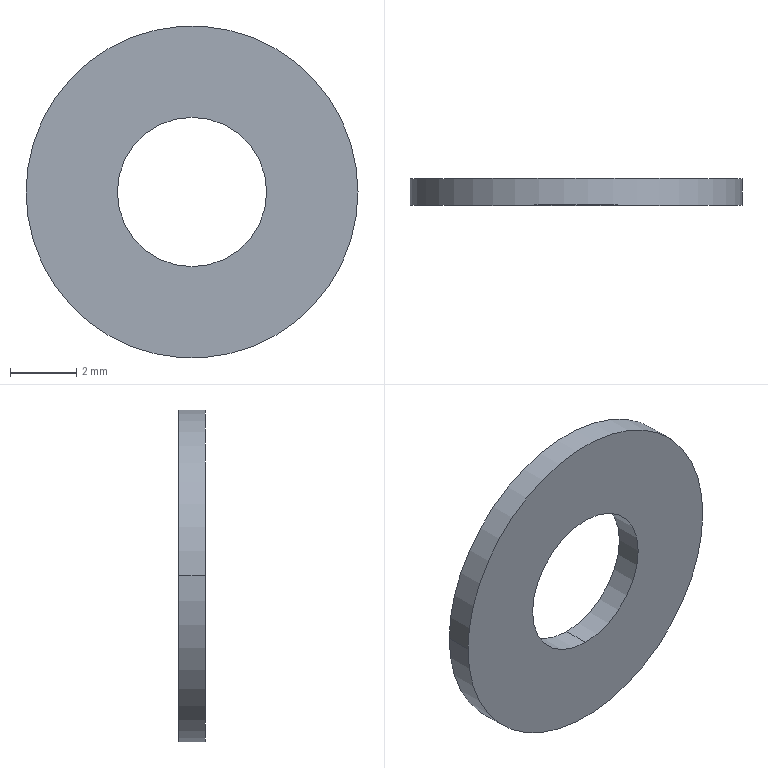Part | STEP file | ZZ21-M4-8 | 1 solid | 6 faces | box 10 x 0.8 x 10 mm | volume 50.108 mm3 | cylinder 4 | plane 2 | commonest cylinder face diameters 4.5 x2 10 x2
STEP:
#1=CARTESIAN_POINT('',(0.,0.,0.));
#2=DIRECTION('',(0.,0.,1.));
#3=DIRECTION('',(1.,0.,0.));
#4=AXIS2_PLACEMENT_3D('',#1,#2,#3);
#5=CARTESIAN_POINT('',(0.,0.,-2.25));
#6=VERTEX_POINT('',#5);
#7=CARTESIAN_POINT('',(0.,0.8,-2.25));
#8=VERTEX_POINT('',#7);
#9=CARTESIAN_POINT('',(0.,0.,-2.25));
#10=DIRECTION('',(0.,1.,0.));
#11=VECTOR('',#10,1.);
#12=LINE('',#9,#11);
#13=CARTESIAN_POINT('',(0.,0.,0.));
#14=DIRECTION('',(0.,1.,0.));
#15=DIRECTION('',(0.,0.,-1.));
#16=AXIS2_PLACEMENT_3D('',#13,#14,#15);
#17=CYLINDRICAL_SURFACE('',#16,2.25);
#18=CARTESIAN_POINT('',(6.283,0.));
#19=DIRECTION('',(0.,1.));
#20=VECTOR('',#19,1.);
#21=LINE('',#18,#20);
#22=(GEOMETRIC_REPRESENTATION_CONTEXT(2)PARAMETRIC_REPRESENTATION_CONTEXT()REPRESENTATION_CONTEXT('',''));
#23=DEFINITIONAL_REPRESENTATION('',(#21),#22);
#24=PCURVE('',#17,#23);
#25=CARTESIAN_POINT('',(0.,0.,0.));
#26=DIRECTION('',(0.,1.,0.));
#27=DIRECTION('',(0.,0.,-1.));
#28=AXIS2_PLACEMENT_3D('',#25,#26,#27);
#29=CYLINDRICAL_SURFACE('',#28,2.25);
#30=CARTESIAN_POINT('',(0.,0.));
#31=DIRECTION('',(0.,1.));
#32=VECTOR('',#31,1.);
#33=LINE('',#30,#32);
#34=(GEOMETRIC_REPRESENTATION_CONTEXT(2)PARAMETRIC_REPRESENTATION_CONTEXT()REPRESENTATION_CONTEXT('',''));
#35=DEFINITIONAL_REPRESENTATION('',(#33),#34);
#36=PCURVE('',#29,#35);
#37=SURFACE_CURVE('',#12,(#24,#36),.PCURVE_S1.);
#38=EDGE_CURVE('',#6,#8,#37,.T.);
#39=ORIENTED_EDGE('',*,*,#38,.T.);
#40=CARTESIAN_POINT('',(0.,0.8,2.25));
#41=VERTEX_POINT('',#40);
#42=CARTESIAN_POINT('',(0.,0.8,0.));
#43=DIRECTION('',(0.,-1.,0.));
#44=DIRECTION('',(0.,0.,1.));
#45=AXIS2_PLACEMENT_3D('',#42,#43,#44);
#46=CIRCLE('',#45,2.25);
#47=CARTESIAN_POINT('',(9.425,0.8));
#48=DIRECTION('',(-1.,0.));
#49=VECTOR('',#48,1.);
#50=LINE('',#47,#49);
#51=(GEOMETRIC_REPRESENTATION_CONTEXT(2)PARAMETRIC_REPRESENTATION_CONTEXT()REPRESENTATION_CONTEXT('',''));
#52=DEFINITIONAL_REPRESENTATION('',(#50),#51);
#53=PCURVE('',#17,#52);
#54=CARTESIAN_POINT('',(0.,0.8,0.));
#55=DIRECTION('',(0.,1.,0.));
#56=DIRECTION('',(-1.,0.,0.));
#57=AXIS2_PLACEMENT_3D('',#54,#55,#56);
#58=PLANE('',#57);
#59=CARTESIAN_POINT('',(0.,2.25));
#60=CARTESIAN_POINT('',(3.897,2.25));
#61=CARTESIAN_POINT('',(1.949,-1.125));
#62=CARTESIAN_POINT('',(0.,-4.5));
#63=CARTESIAN_POINT('',(-1.949,-1.125));
#64=CARTESIAN_POINT('',(-3.897,2.25));
#65=CARTESIAN_POINT('',(0.,2.25));
#66=(BOUNDED_CURVE()B_SPLINE_CURVE(2,(#59,#60,#61,#62,#63,#64,#65),.UNSPECIFIED.,.T.,.F.)B_SPLINE_CURVE_WITH_KNOTS((1,2,2,2,2,1),(-2.094,0.,2.094,4.189,6.283,8.378),.UNSPECIFIED.)CURVE()GEOMETRIC_REPRESENTATION_ITEM()RATIONAL_B_SPLINE_CURVE((1.,0.5,1.,0.5,1.,0.5,1.))REPRESENTATION_ITEM(''));
#67=(GEOMETRIC_REPRESENTATION_CONTEXT(2)PARAMETRIC_REPRESENTATION_CONTEXT()REPRESENTATION_CONTEXT('',''));
#68=DEFINITIONAL_REPRESENTATION('',(#66),#67);
#69=PCURVE('',#58,#68);
#70=SURFACE_CURVE('',#46,(#53,#69),.PCURVE_S1.);
#71=EDGE_CURVE('',#8,#41,#70,.T.);
#72=ORIENTED_EDGE('',*,*,#71,.T.);
#73=CARTESIAN_POINT('',(0.,0.,2.25));
#74=VERTEX_POINT('',#73);
#75=CARTESIAN_POINT('',(0.,0.,2.25));
#76=DIRECTION('',(0.,1.,0.));
#77=VECTOR('',#76,1.);
#78=LINE('',#75,#77);
#79=CARTESIAN_POINT('',(3.142,0.));
#80=DIRECTION('',(0.,1.));
#81=VECTOR('',#80,1.);
#82=LINE('',#79,#81);
#83=(GEOMETRIC_REPRESENTATION_CONTEXT(2)PARAMETRIC_REPRESENTATION_CONTEXT()REPRESENTATION_CONTEXT('',''));
#84=DEFINITIONAL_REPRESENTATION('',(#82),#83);
#85=PCURVE('',#17,#84);
#86=CARTESIAN_POINT('',(3.142,0.));
#87=DIRECTION('',(0.,1.));
#88=VECTOR('',#87,1.);
#89=LINE('',#86,#88);
#90=(GEOMETRIC_REPRESENTATION_CONTEXT(2)PARAMETRIC_REPRESENTATION_CONTEXT()REPRESENTATION_CONTEXT('',''));
#91=DEFINITIONAL_REPRESENTATION('',(#89),#90);
#92=PCURVE('',#29,#91);
#93=SURFACE_CURVE('',#78,(#85,#92),.PCURVE_S1.);
#94=EDGE_CURVE('',#74,#41,#93,.T.);
#95=ORIENTED_EDGE('',*,*,#94,.F.);
#96=CARTESIAN_POINT('',(0.,0.,0.));
#97=DIRECTION('',(0.,1.,0.));
#98=DIRECTION('',(0.,0.,-1.));
#99=AXIS2_PLACEMENT_3D('',#96,#97,#98);
#100=CIRCLE('',#99,2.25);
#101=CARTESIAN_POINT('',(0.,0.));
#102=DIRECTION('',(1.,0.));
#103=VECTOR('',#102,1.);
#104=LINE('',#101,#103);
#105=(GEOMETRIC_REPRESENTATION_CONTEXT(2)PARAMETRIC_REPRESENTATION_CONTEXT()REPRESENTATION_CONTEXT('',''));
#106=DEFINITIONAL_REPRESENTATION('',(#104),#105);
#107=PCURVE('',#17,#106);
#108=CARTESIAN_POINT('',(0.,0.,0.));
#109=DIRECTION('',(0.,-1.,0.));
#110=DIRECTION('',(1.,0.,0.));
#111=AXIS2_PLACEMENT_3D('',#108,#109,#110);
#112=PLANE('',#111);
#113=CARTESIAN_POINT('',(0.,-2.25));
#114=CARTESIAN_POINT('',(-3.897,-2.25));
#115=CARTESIAN_POINT('',(-1.949,1.125));
#116=CARTESIAN_POINT('',(0.,4.5));
#117=CARTESIAN_POINT('',(1.949,1.125));
#118=CARTESIAN_POINT('',(3.897,-2.25));
#119=CARTESIAN_POINT('',(0.,-2.25));
#120=(BOUNDED_CURVE()B_SPLINE_CURVE(2,(#113,#114,#115,#116,#117,#118,#119),.UNSPECIFIED.,.T.,.F.)B_SPLINE_CURVE_WITH_KNOTS((1,2,2,2,2,1),(-2.094,0.,2.094,4.189,6.283,8.378),.UNSPECIFIED.)CURVE()GEOMETRIC_REPRESENTATION_ITEM()RATIONAL_B_SPLINE_CURVE((1.,0.5,1.,0.5,1.,0.5,1.))REPRESENTATION_ITEM(''));
#121=(GEOMETRIC_REPRESENTATION_CONTEXT(2)PARAMETRIC_REPRESENTATION_CONTEXT()REPRESENTATION_CONTEXT('',''));
#122=DEFINITIONAL_REPRESENTATION('',(#120),#121);
#123=PCURVE('',#112,#122);
#124=SURFACE_CURVE('',#100,(#107,#123),.PCURVE_S1.);
#125=EDGE_CURVE('',#74,#6,#124,.T.);
#126=ORIENTED_EDGE('',*,*,#125,.T.);
#127=EDGE_LOOP('',(#39,#72,#95,#126));
#128=FACE_BOUND('',#127,.F.);
#129=ADVANCED_FACE('',(#128),#17,.F.);
#130=CARTESIAN_POINT('',(-5.,0.,0.));
#131=VERTEX_POINT('',#130);
#132=CARTESIAN_POINT('',(5.,0.,0.));
#133=VERTEX_POINT('',#132);
#134=CARTESIAN_POINT('',(0.,0.,0.));
#135=DIRECTION('',(0.,1.,0.));
#136=DIRECTION('',(-1.,0.,0.));
#137=AXIS2_PLACEMENT_3D('',#134,#135,#136);
#138=CIRCLE('',#137,5.);
#139=CARTESIAN_POINT('',(0.,0.,0.));
#140=DIRECTION('',(0.,1.,0.));
#141=DIRECTION('',(-1.,0.,0.));
#142=AXIS2_PLACEMENT_3D('',#139,#140,#141);
#143=CYLINDRICAL_SURFACE('',#142,5.);
#144=CARTESIAN_POINT('',(0.,0.));
#145=DIRECTION('',(1.,0.));
#146=VECTOR('',#145,1.);
#147=LINE('',#144,#146);
#148=(GEOMETRIC_REPRESENTATION_CONTEXT(2)PARAMETRIC_REPRESENTATION_CONTEXT()REPRESENTATION_CONTEXT('',''));
#149=DEFINITIONAL_REPRESENTATION('',(#147),#148);
#150=PCURVE('',#143,#149);
#151=CARTESIAN_POINT('',(-5.,0.));
#152=CARTESIAN_POINT('',(-5.,8.66));
#153=CARTESIAN_POINT('',(2.5,4.33));
#154=CARTESIAN_POINT('',(10.,0.));
#155=CARTESIAN_POINT('',(2.5,-4.33));
#156=CARTESIAN_POINT('',(-5.,-8.66));
#157=CARTESIAN_POINT('',(-5.,0.));
#158=(BOUNDED_CURVE()B_SPLINE_CURVE(2,(#151,#152,#153,#154,#155,#156,#157),.UNSPECIFIED.,.T.,.F.)B_SPLINE_CURVE_WITH_KNOTS((1,2,2,2,2,1),(-2.094,0.,2.094,4.189,6.283,8.378),.UNSPECIFIED.)CURVE()GEOMETRIC_REPRESENTATION_ITEM()RATIONAL_B_SPLINE_CURVE((1.,0.5,1.,0.5,1.,0.5,1.))REPRESENTATION_ITEM(''));
#159=(GEOMETRIC_REPRESENTATION_CONTEXT(2)PARAMETRIC_REPRESENTATION_CONTEXT()REPRESENTATION_CONTEXT('',''));
#160=DEFINITIONAL_REPRESENTATION('',(#158),#159);
#161=PCURVE('',#112,#160);
#162=SURFACE_CURVE('',#138,(#150,#161),.PCURVE_S1.);
#163=EDGE_CURVE('',#131,#133,#162,.T.);
#164=ORIENTED_EDGE('',*,*,#163,.T.);
#165=CARTESIAN_POINT('',(5.,0.8,0.));
#166=VERTEX_POINT('',#165);
#167=CARTESIAN_POINT('',(5.,0.,0.));
#168=DIRECTION('',(0.,1.,0.));
#169=VECTOR('',#168,1.);
#170=LINE('',#167,#169);
#171=CARTESIAN_POINT('',(3.142,0.));
#172=DIRECTION('',(0.,1.));
#173=VECTOR('',#172,1.);
#174=LINE('',#171,#173);
#175=(GEOMETRIC_REPRESENTATION_CONTEXT(2)PARAMETRIC_REPRESENTATION_CONTEXT()REPRESENTATION_CONTEXT('',''));
#176=DEFINITIONAL_REPRESENTATION('',(#174),#175);
#177=PCURVE('',#143,#176);
#178=CARTESIAN_POINT('',(0.,0.,0.));
#179=DIRECTION('',(0.,1.,0.));
#180=DIRECTION('',(-1.,0.,0.));
#181=AXIS2_PLACEMENT_3D('',#178,#179,#180);
#182=CYLINDRICAL_SURFACE('',#181,5.);
#183=CARTESIAN_POINT('',(3.142,0.));
#184=DIRECTION('',(0.,1.));
#185=VECTOR('',#184,1.);
#186=LINE('',#183,#185);
#187=(GEOMETRIC_REPRESENTATION_CONTEXT(2)PARAMETRIC_REPRESENTATION_CONTEXT()REPRESENTATION_CONTEXT('',''));
#188=DEFINITIONAL_REPRESENTATION('',(#186),#187);
#189=PCURVE('',#182,#188);
#190=SURFACE_CURVE('',#170,(#177,#189),.PCURVE_S1.);
#191=EDGE_CURVE('',#133,#166,#190,.T.);
#192=ORIENTED_EDGE('',*,*,#191,.T.);
#193=CARTESIAN_POINT('',(-5.,0.8,0.));
#194=VERTEX_POINT('',#193);
#195=CARTESIAN_POINT('',(0.,0.8,0.));
#196=DIRECTION('',(0.,-1.,0.));
#197=DIRECTION('',(1.,0.,0.));
#198=AXIS2_PLACEMENT_3D('',#195,#196,#197);
#199=CIRCLE('',#198,5.);
#200=CARTESIAN_POINT('',(3.142,0.8));
#201=DIRECTION('',(-1.,0.));
#202=VECTOR('',#201,1.);
#203=LINE('',#200,#202);
#204=(GEOMETRIC_REPRESENTATION_CONTEXT(2)PARAMETRIC_REPRESENTATION_CONTEXT()REPRESENTATION_CONTEXT('',''));
#205=DEFINITIONAL_REPRESENTATION('',(#203),#204);
#206=PCURVE('',#143,#205);
#207=CARTESIAN_POINT('',(-5.,0.));
#208=CARTESIAN_POINT('',(-5.,8.66));
#209=CARTESIAN_POINT('',(2.5,4.33));
#210=CARTESIAN_POINT('',(10.,0.));
#211=CARTESIAN_POINT('',(2.5,-4.33));
#212=CARTESIAN_POINT('',(-5.,-8.66));
#213=CARTESIAN_POINT('',(-5.,0.));
#214=(BOUNDED_CURVE()B_SPLINE_CURVE(2,(#207,#208,#209,#210,#211,#212,#213),.UNSPECIFIED.,.T.,.F.)B_SPLINE_CURVE_WITH_KNOTS((1,2,2,2,2,1),(-2.094,0.,2.094,4.189,6.283,8.378),.UNSPECIFIED.)CURVE()GEOMETRIC_REPRESENTATION_ITEM()RATIONAL_B_SPLINE_CURVE((1.,0.5,1.,0.5,1.,0.5,1.))REPRESENTATION_ITEM(''));
#215=(GEOMETRIC_REPRESENTATION_CONTEXT(2)PARAMETRIC_REPRESENTATION_CONTEXT()REPRESENTATION_CONTEXT('',''));
#216=DEFINITIONAL_REPRESENTATION('',(#214),#215);
#217=PCURVE('',#58,#216);
#218=SURFACE_CURVE('',#199,(#206,#217),.PCURVE_S1.);
#219=EDGE_CURVE('',#166,#194,#218,.T.);
#220=ORIENTED_EDGE('',*,*,#219,.T.);
#221=CARTESIAN_POINT('',(-5.,0.,0.));
#222=DIRECTION('',(0.,1.,0.));
#223=VECTOR('',#222,1.);
#224=LINE('',#221,#223);
#225=CARTESIAN_POINT('',(0.,0.));
#226=DIRECTION('',(0.,1.));
#227=VECTOR('',#226,1.);
#228=LINE('',#225,#227);
#229=(GEOMETRIC_REPRESENTATION_CONTEXT(2)PARAMETRIC_REPRESENTATION_CONTEXT()REPRESENTATION_CONTEXT('',''));
#230=DEFINITIONAL_REPRESENTATION('',(#228),#229);
#231=PCURVE('',#143,#230);
#232=CARTESIAN_POINT('',(6.283,0.));
#233=DIRECTION('',(0.,1.));
#234=VECTOR('',#233,1.);
#235=LINE('',#232,#234);
#236=(GEOMETRIC_REPRESENTATION_CONTEXT(2)PARAMETRIC_REPRESENTATION_CONTEXT()REPRESENTATION_CONTEXT('',''));
#237=DEFINITIONAL_REPRESENTATION('',(#235),#236);
#238=PCURVE('',#182,#237);
#239=SURFACE_CURVE('',#224,(#231,#238),.PCURVE_S1.);
#240=EDGE_CURVE('',#131,#194,#239,.T.);
#241=ORIENTED_EDGE('',*,*,#240,.F.);
#242=EDGE_LOOP('',(#164,#192,#220,#241));
#243=FACE_BOUND('',#242,.T.);
#244=ADVANCED_FACE('',(#243),#143,.T.);
#245=ORIENTED_EDGE('',*,*,#71,.T.);
#246=CARTESIAN_POINT('',(0.,0.8,0.));
#247=DIRECTION('',(0.,-1.,0.));
#248=DIRECTION('',(0.,0.,1.));
#249=AXIS2_PLACEMENT_3D('',#246,#247,#248);
#250=CIRCLE('',#249,2.25);
#251=CARTESIAN_POINT('',(0.,2.25));
#252=CARTESIAN_POINT('',(3.897,2.25));
#253=CARTESIAN_POINT('',(1.949,-1.125));
#254=CARTESIAN_POINT('',(0.,-4.5));
#255=CARTESIAN_POINT('',(-1.949,-1.125));
#256=CARTESIAN_POINT('',(-3.897,2.25));
#257=CARTESIAN_POINT('',(0.,2.25));
#258=(BOUNDED_CURVE()B_SPLINE_CURVE(2,(#251,#252,#253,#254,#255,#256,#257),.UNSPECIFIED.,.T.,.F.)B_SPLINE_CURVE_WITH_KNOTS((1,2,2,2,2,1),(-2.094,0.,2.094,4.189,6.283,8.378),.UNSPECIFIED.)CURVE()GEOMETRIC_REPRESENTATION_ITEM()RATIONAL_B_SPLINE_CURVE((1.,0.5,1.,0.5,1.,0.5,1.))REPRESENTATION_ITEM(''));
#259=(GEOMETRIC_REPRESENTATION_CONTEXT(2)PARAMETRIC_REPRESENTATION_CONTEXT()REPRESENTATION_CONTEXT('',''));
#260=DEFINITIONAL_REPRESENTATION('',(#258),#259);
#261=PCURVE('',#58,#260);
#262=CARTESIAN_POINT('',(3.142,0.8));
#263=DIRECTION('',(-1.,0.));
#264=VECTOR('',#263,1.);
#265=LINE('',#262,#264);
#266=(GEOMETRIC_REPRESENTATION_CONTEXT(2)PARAMETRIC_REPRESENTATION_CONTEXT()REPRESENTATION_CONTEXT('',''));
#267=DEFINITIONAL_REPRESENTATION('',(#265),#266);
#268=PCURVE('',#29,#267);
#269=SURFACE_CURVE('',#250,(#261,#268),.PCURVE_S1.);
#270=EDGE_CURVE('',#41,#8,#269,.T.);
#271=ORIENTED_EDGE('',*,*,#270,.T.);
#272=EDGE_LOOP('',(#245,#271));
#273=FACE_BOUND('',#272,.T.);
#274=CARTESIAN_POINT('',(0.,0.8,0.));
#275=DIRECTION('',(0.,-1.,0.));
#276=DIRECTION('',(1.,0.,0.));
#277=AXIS2_PLACEMENT_3D('',#274,#275,#276);
#278=CIRCLE('',#277,5.);
#279=CARTESIAN_POINT('',(-5.,0.));
#280=CARTESIAN_POINT('',(-5.,8.66));
#281=CARTESIAN_POINT('',(2.5,4.33));
#282=CARTESIAN_POINT('',(10.,0.));
#283=CARTESIAN_POINT('',(2.5,-4.33));
#284=CARTESIAN_POINT('',(-5.,-8.66));
#285=CARTESIAN_POINT('',(-5.,0.));
#286=(BOUNDED_CURVE()B_SPLINE_CURVE(2,(#279,#280,#281,#282,#283,#284,#285),.UNSPECIFIED.,.T.,.F.)B_SPLINE_CURVE_WITH_KNOTS((1,2,2,2,2,1),(-2.094,0.,2.094,4.189,6.283,8.378),.UNSPECIFIED.)CURVE()GEOMETRIC_REPRESENTATION_ITEM()RATIONAL_B_SPLINE_CURVE((1.,0.5,1.,0.5,1.,0.5,1.))REPRESENTATION_ITEM(''));
#287=(GEOMETRIC_REPRESENTATION_CONTEXT(2)PARAMETRIC_REPRESENTATION_CONTEXT()REPRESENTATION_CONTEXT('',''));
#288=DEFINITIONAL_REPRESENTATION('',(#286),#287);
#289=PCURVE('',#58,#288);
#290=CARTESIAN_POINT('',(9.425,0.8));
#291=DIRECTION('',(-1.,0.));
#292=VECTOR('',#291,1.);
#293=LINE('',#290,#292);
#294=(GEOMETRIC_REPRESENTATION_CONTEXT(2)PARAMETRIC_REPRESENTATION_CONTEXT()REPRESENTATION_CONTEXT('',''));
#295=DEFINITIONAL_REPRESENTATION('',(#293),#294);
#296=PCURVE('',#182,#295);
#297=SURFACE_CURVE('',#278,(#289,#296),.PCURVE_S1.);
#298=EDGE_CURVE('',#194,#166,#297,.T.);
#299=ORIENTED_EDGE('',*,*,#298,.F.);
#300=ORIENTED_EDGE('',*,*,#219,.F.);
#301=EDGE_LOOP('',(#299,#300));
#302=FACE_BOUND('',#301,.T.);
#303=ADVANCED_FACE('',(#273,#302),#58,.T.);
#304=CARTESIAN_POINT('',(0.,0.,0.));
#305=DIRECTION('',(0.,1.,0.));
#306=DIRECTION('',(0.,0.,-1.));
#307=AXIS2_PLACEMENT_3D('',#304,#305,#306);
#308=CIRCLE('',#307,2.25);
#309=CARTESIAN_POINT('',(0.,-2.25));
#310=CARTESIAN_POINT('',(-3.897,-2.25));
#311=CARTESIAN_POINT('',(-1.949,1.125));
#312=CARTESIAN_POINT('',(0.,4.5));
#313=CARTESIAN_POINT('',(1.949,1.125));
#314=CARTESIAN_POINT('',(3.897,-2.25));
#315=CARTESIAN_POINT('',(0.,-2.25));
#316=(BOUNDED_CURVE()B_SPLINE_CURVE(2,(#309,#310,#311,#312,#313,#314,#315),.UNSPECIFIED.,.T.,.F.)B_SPLINE_CURVE_WITH_KNOTS((1,2,2,2,2,1),(-2.094,0.,2.094,4.189,6.283,8.378),.UNSPECIFIED.)CURVE()GEOMETRIC_REPRESENTATION_ITEM()RATIONAL_B_SPLINE_CURVE((1.,0.5,1.,0.5,1.,0.5,1.))REPRESENTATION_ITEM(''));
#317=(GEOMETRIC_REPRESENTATION_CONTEXT(2)PARAMETRIC_REPRESENTATION_CONTEXT()REPRESENTATION_CONTEXT('',''));
#318=DEFINITIONAL_REPRESENTATION('',(#316),#317);
#319=PCURVE('',#112,#318);
#320=CARTESIAN_POINT('',(0.,0.));
#321=DIRECTION('',(1.,0.));
#322=VECTOR('',#321,1.);
#323=LINE('',#320,#322);
#324=(GEOMETRIC_REPRESENTATION_CONTEXT(2)PARAMETRIC_REPRESENTATION_CONTEXT()REPRESENTATION_CONTEXT('',''));
#325=DEFINITIONAL_REPRESENTATION('',(#323),#324);
#326=PCURVE('',#29,#325);
#327=SURFACE_CURVE('',#308,(#319,#326),.PCURVE_S1.);
#328=EDGE_CURVE('',#6,#74,#327,.T.);
#329=ORIENTED_EDGE('',*,*,#328,.T.);
#330=ORIENTED_EDGE('',*,*,#125,.T.);
#331=EDGE_LOOP('',(#329,#330));
#332=FACE_BOUND('',#331,.T.);
#333=ORIENTED_EDGE('',*,*,#163,.F.);
#334=CARTESIAN_POINT('',(0.,0.,0.));
#335=DIRECTION('',(0.,1.,0.));
#336=DIRECTION('',(-1.,0.,0.));
#337=AXIS2_PLACEMENT_3D('',#334,#335,#336);
#338=CIRCLE('',#337,5.);
#339=CARTESIAN_POINT('',(-5.,0.));
#340=CARTESIAN_POINT('',(-5.,8.66));
#341=CARTESIAN_POINT('',(2.5,4.33));
#342=CARTESIAN_POINT('',(10.,0.));
#343=CARTESIAN_POINT('',(2.5,-4.33));
#344=CARTESIAN_POINT('',(-5.,-8.66));
#345=CARTESIAN_POINT('',(-5.,0.));
#346=(BOUNDED_CURVE()B_SPLINE_CURVE(2,(#339,#340,#341,#342,#343,#344,#345),.UNSPECIFIED.,.T.,.F.)B_SPLINE_CURVE_WITH_KNOTS((1,2,2,2,2,1),(-2.094,0.,2.094,4.189,6.283,8.378),.UNSPECIFIED.)CURVE()GEOMETRIC_REPRESENTATION_ITEM()RATIONAL_B_SPLINE_CURVE((1.,0.5,1.,0.5,1.,0.5,1.))REPRESENTATION_ITEM(''));
#347=(GEOMETRIC_REPRESENTATION_CONTEXT(2)PARAMETRIC_REPRESENTATION_CONTEXT()REPRESENTATION_CONTEXT('',''));
#348=DEFINITIONAL_REPRESENTATION('',(#346),#347);
#349=PCURVE('',#112,#348);
#350=CARTESIAN_POINT('',(0.,0.));
#351=DIRECTION('',(1.,0.));
#352=VECTOR('',#351,1.);
#353=LINE('',#350,#352);
#354=(GEOMETRIC_REPRESENTATION_CONTEXT(2)PARAMETRIC_REPRESENTATION_CONTEXT()REPRESENTATION_CONTEXT('',''));
#355=DEFINITIONAL_REPRESENTATION('',(#353),#354);
#356=PCURVE('',#182,#355);
#357=SURFACE_CURVE('',#338,(#349,#356),.PCURVE_S1.);
#358=EDGE_CURVE('',#133,#131,#357,.T.);
#359=ORIENTED_EDGE('',*,*,#358,.F.);
#360=EDGE_LOOP('',(#333,#359));
#361=FACE_BOUND('',#360,.T.);
#362=ADVANCED_FACE('',(#332,#361),#112,.T.);
#363=ORIENTED_EDGE('',*,*,#191,.F.);
#364=ORIENTED_EDGE('',*,*,#358,.T.);
#365=ORIENTED_EDGE('',*,*,#240,.T.);
#366=ORIENTED_EDGE('',*,*,#298,.T.);
#367=EDGE_LOOP('',(#363,#364,#365,#366));
#368=FACE_BOUND('',#367,.T.);
#369=ADVANCED_FACE('',(#368),#182,.T.);
#370=ORIENTED_EDGE('',*,*,#270,.T.);
#371=ORIENTED_EDGE('',*,*,#38,.F.);
#372=ORIENTED_EDGE('',*,*,#328,.T.);
#373=ORIENTED_EDGE('',*,*,#94,.T.);
#374=EDGE_LOOP('',(#370,#371,#372,#373));
#375=FACE_BOUND('',#374,.F.);
#376=ADVANCED_FACE('',(#375),#29,.F.);
#377=CLOSED_SHELL('',(#129,#244,#303,#362,#369,#376));
#378=MANIFOLD_SOLID_BREP('',#377);
#379=(LENGTH_UNIT()NAMED_UNIT(*)SI_UNIT(.MILLI.,.METRE.));
#380=UNCERTAINTY_MEASURE_WITH_UNIT(LENGTH_MEASURE(0.0000001),#379,'','');
#381=(NAMED_UNIT(*)PLANE_ANGLE_UNIT()SI_UNIT($,.RADIAN.));
#382=(NAMED_UNIT(*)SI_UNIT($,.STERADIAN.)SOLID_ANGLE_UNIT());
#383=(GEOMETRIC_REPRESENTATION_CONTEXT(3)GLOBAL_UNCERTAINTY_ASSIGNED_CONTEXT((#380))GLOBAL_UNIT_ASSIGNED_CONTEXT((#379,#381,#382))REPRESENTATION_CONTEXT('',''));
#384=ADVANCED_BREP_SHAPE_REPRESENTATION('',(#4,#378),#383);